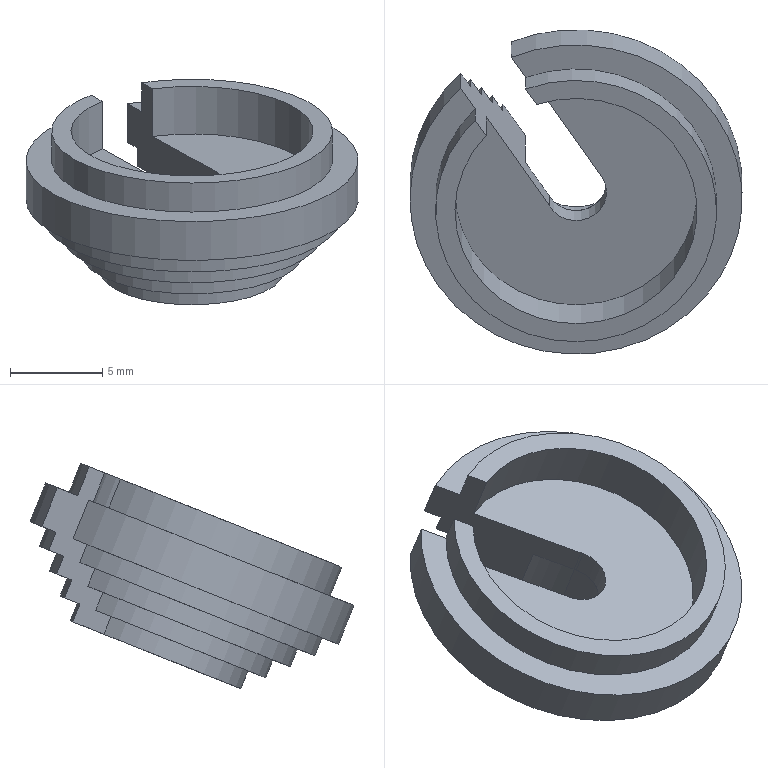Part | STEP file | Cut-Extrude7 | 1 solid | 26 faces | box 18 x 17.564 x 12.214 mm | volume 867.182 mm3 | cylinder 12 | plane 10 | spline 2 | cone 2 | commonest cylinder face diameters 3.3 x2 5.96 x2 16.1 x2 9.96 x1 12 x1 13.12 x1